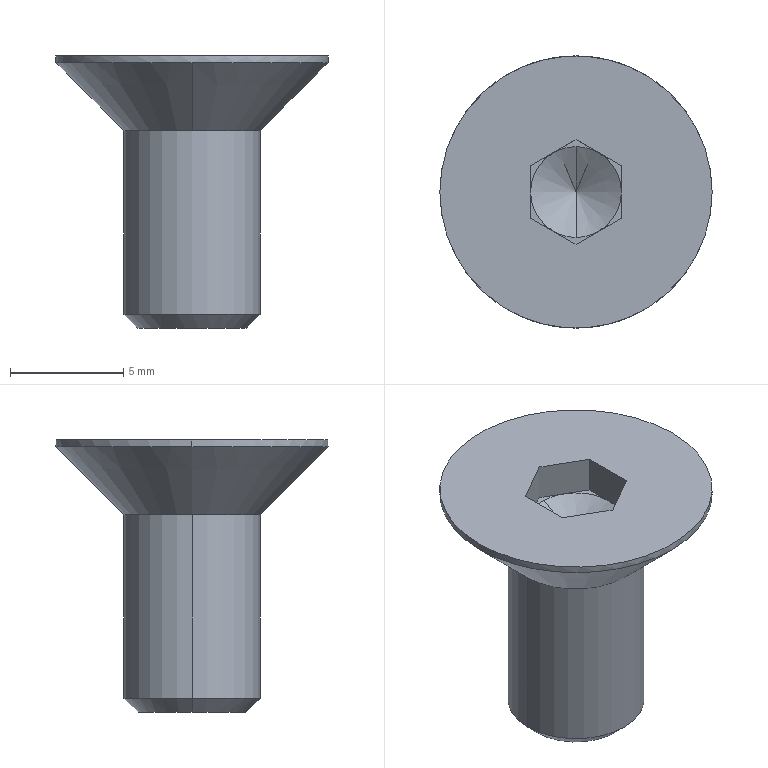Part | SolidWorks | features BaseBody 1 | 1 solid | 24 faces | box 12 x 12 x 12 mm | volume 446.831 mm3 | plane 14 | cone 6 | cylinder 4 | commonest cylinder face diameters 6 x2 12 x2
STEP:
#1=CARTESIAN_POINT('',(0.,6.,3.));
#2=VERTEX_POINT('',#1);
#3=CARTESIAN_POINT('',(-6.,0.,3.));
#4=VERTEX_POINT('',#3);
#5=CARTESIAN_POINT('',(0.,0.,3.));
#6=DIRECTION('',(0.,0.,1.));
#7=DIRECTION('',(1.,0.,0.));
#8=AXIS2_PLACEMENT_3D('',#5,#6,#7);
#9=CIRCLE('',#8,6.);
#10=EDGE_CURVE('',#2,#4,#9,.T.);
#11=ORIENTED_EDGE('',*,*,#10,.T.);
#12=CARTESIAN_POINT('',(-6.,0.,3.3));
#13=VERTEX_POINT('',#12);
#14=CARTESIAN_POINT('',(-6.,0.,0.));
#15=DIRECTION('',(0.,0.,1.));
#16=VECTOR('',#15,1000.);
#17=LINE('',#14,#16);
#18=EDGE_CURVE('',#4,#13,#17,.T.);
#19=ORIENTED_EDGE('',*,*,#18,.T.);
#20=CARTESIAN_POINT('',(6.,0.,3.3));
#21=VERTEX_POINT('',#20);
#22=CARTESIAN_POINT('',(0.,0.,3.3));
#23=DIRECTION('',(0.,0.,-1.));
#24=DIRECTION('',(1.,0.,0.));
#25=AXIS2_PLACEMENT_3D('',#22,#23,#24);
#26=CIRCLE('',#25,6.);
#27=EDGE_CURVE('',#13,#21,#26,.T.);
#28=ORIENTED_EDGE('',*,*,#27,.T.);
#29=CARTESIAN_POINT('',(6.,0.,3.));
#30=VERTEX_POINT('',#29);
#31=CARTESIAN_POINT('',(6.,0.,0.));
#32=DIRECTION('',(0.,0.,1.));
#33=VECTOR('',#32,1000.);
#34=LINE('',#31,#33);
#35=EDGE_CURVE('',#30,#21,#34,.T.);
#36=ORIENTED_EDGE('',*,*,#35,.F.);
#37=CARTESIAN_POINT('',(0.,0.,3.));
#38=DIRECTION('',(0.,0.,1.));
#39=DIRECTION('',(1.,0.,0.));
#40=AXIS2_PLACEMENT_3D('',#37,#38,#39);
#41=CIRCLE('',#40,6.);
#42=EDGE_CURVE('',#30,#2,#41,.T.);
#43=ORIENTED_EDGE('',*,*,#42,.T.);
#44=EDGE_LOOP('',(#11,#19,#28,#36,#43));
#45=FACE_OUTER_BOUND('',#44,.T.);
#46=CARTESIAN_POINT('',(0.,0.,0.));
#47=DIRECTION('',(0.,0.,1.));
#48=DIRECTION('',(1.,0.,0.));
#49=AXIS2_PLACEMENT_3D('',#46,#47,#48);
#50=CYLINDRICAL_SURFACE('',#49,6.);
#51=ADVANCED_FACE('',(#45),#50,.T.);
#52=CARTESIAN_POINT('',(3.,0.,0.));
#53=VERTEX_POINT('',#52);
#54=CARTESIAN_POINT('',(0.,3.,0.));
#55=VERTEX_POINT('',#54);
#56=CARTESIAN_POINT('',(0.,0.,0.));
#57=DIRECTION('',(0.,0.,1.));
#58=DIRECTION('',(1.,0.,0.));
#59=AXIS2_PLACEMENT_3D('',#56,#57,#58);
#60=CIRCLE('',#59,3.);
#61=EDGE_CURVE('',#53,#55,#60,.T.);
#62=ORIENTED_EDGE('',*,*,#61,.T.);
#63=CARTESIAN_POINT('',(0.,6.,3.));
#64=DIRECTION('',(0.,0.7071,0.7071));
#65=VECTOR('',#64,1000.);
#66=LINE('',#63,#65);
#67=EDGE_CURVE('',#55,#2,#66,.T.);
#68=ORIENTED_EDGE('',*,*,#67,.T.);
#69=ORIENTED_EDGE('',*,*,#42,.F.);
#70=CARTESIAN_POINT('',(0.,-6.,3.));
#71=VERTEX_POINT('',#70);
#72=CARTESIAN_POINT('',(0.,0.,3.));
#73=DIRECTION('',(0.,0.,1.));
#74=DIRECTION('',(1.,0.,0.));
#75=AXIS2_PLACEMENT_3D('',#72,#73,#74);
#76=CIRCLE('',#75,6.);
#77=EDGE_CURVE('',#71,#30,#76,.T.);
#78=ORIENTED_EDGE('',*,*,#77,.F.);
#79=CARTESIAN_POINT('',(0.,-3.,0.));
#80=VERTEX_POINT('',#79);
#81=CARTESIAN_POINT('',(0.,-6.,3.));
#82=DIRECTION('',(0.,-0.7071,0.7071));
#83=VECTOR('',#82,1000.);
#84=LINE('',#81,#83);
#85=EDGE_CURVE('',#80,#71,#84,.T.);
#86=ORIENTED_EDGE('',*,*,#85,.F.);
#87=CARTESIAN_POINT('',(0.,0.,0.));
#88=DIRECTION('',(0.,0.,1.));
#89=DIRECTION('',(1.,0.,0.));
#90=AXIS2_PLACEMENT_3D('',#87,#88,#89);
#91=CIRCLE('',#90,3.);
#92=EDGE_CURVE('',#80,#53,#91,.T.);
#93=ORIENTED_EDGE('',*,*,#92,.T.);
#94=EDGE_LOOP('',(#62,#68,#69,#78,#86,#93));
#95=FACE_OUTER_BOUND('',#94,.T.);
#96=CARTESIAN_POINT('',(0.,0.,3.));
#97=DIRECTION('',(0.,0.,1.));
#98=DIRECTION('',(0.,-1.,0.));
#99=AXIS2_PLACEMENT_3D('',#96,#97,#98);
#100=CONICAL_SURFACE('',#99,6.,0.7854);
#101=ADVANCED_FACE('',(#95),#100,.T.);
#102=CARTESIAN_POINT('',(3.,0.,-8.086));
#103=VERTEX_POINT('',#102);
#104=CARTESIAN_POINT('',(-3.,0.,-8.086));
#105=VERTEX_POINT('',#104);
#106=CARTESIAN_POINT('',(0.,0.,-8.086));
#107=DIRECTION('',(0.,0.,1.));
#108=DIRECTION('',(1.,0.,0.));
#109=AXIS2_PLACEMENT_3D('',#106,#107,#108);
#110=CIRCLE('',#109,3.);
#111=EDGE_CURVE('',#103,#105,#110,.T.);
#112=ORIENTED_EDGE('',*,*,#111,.T.);
#113=CARTESIAN_POINT('',(-3.,0.,0.));
#114=VERTEX_POINT('',#113);
#115=CARTESIAN_POINT('',(-3.,0.,-8.7));
#116=DIRECTION('',(0.,0.,1.));
#117=VECTOR('',#116,1000.);
#118=LINE('',#115,#117);
#119=EDGE_CURVE('',#105,#114,#118,.T.);
#120=ORIENTED_EDGE('',*,*,#119,.T.);
#121=CARTESIAN_POINT('',(0.,0.,0.));
#122=DIRECTION('',(0.,0.,1.));
#123=DIRECTION('',(1.,0.,0.));
#124=AXIS2_PLACEMENT_3D('',#121,#122,#123);
#125=CIRCLE('',#124,3.);
#126=EDGE_CURVE('',#55,#114,#125,.T.);
#127=ORIENTED_EDGE('',*,*,#126,.F.);
#128=ORIENTED_EDGE('',*,*,#61,.F.);
#129=CARTESIAN_POINT('',(3.,0.,-8.7));
#130=DIRECTION('',(0.,0.,1.));
#131=VECTOR('',#130,1000.);
#132=LINE('',#129,#131);
#133=EDGE_CURVE('',#103,#53,#132,.T.);
#134=ORIENTED_EDGE('',*,*,#133,.F.);
#135=EDGE_LOOP('',(#112,#120,#127,#128,#134));
#136=FACE_OUTER_BOUND('',#135,.T.);
#137=CARTESIAN_POINT('',(0.,0.,-8.7));
#138=DIRECTION('',(0.,0.,1.));
#139=DIRECTION('',(1.,0.,0.));
#140=AXIS2_PLACEMENT_3D('',#137,#138,#139);
#141=CYLINDRICAL_SURFACE('',#140,3.);
#142=ADVANCED_FACE('',(#136),#141,.T.);
#143=CARTESIAN_POINT('',(0.,0.,0.4953));
#144=VERTEX_POINT('',#143);
#145=CARTESIAN_POINT('',(0.,-2.,1.65));
#146=VERTEX_POINT('',#145);
#147=CARTESIAN_POINT('',(0.,-2.,1.65));
#148=DIRECTION('',(0.,-0.866,0.5));
#149=VECTOR('',#148,1000.);
#150=LINE('',#147,#149);
#151=EDGE_CURVE('',#144,#146,#150,.T.);
#152=ORIENTED_EDGE('',*,*,#151,.F.);
#153=CARTESIAN_POINT('',(0.,2.,1.65));
#154=VERTEX_POINT('',#153);
#155=CARTESIAN_POINT('',(0.,2.,1.65));
#156=DIRECTION('',(0.,0.866,0.5));
#157=VECTOR('',#156,1000.);
#158=LINE('',#155,#157);
#159=EDGE_CURVE('',#144,#154,#158,.T.);
#160=ORIENTED_EDGE('',*,*,#159,.T.);
#161=CARTESIAN_POINT('',(-1.,1.732,1.65));
#162=VERTEX_POINT('',#161);
#163=CARTESIAN_POINT('',(0.,0.,1.65));
#164=DIRECTION('',(0.,0.,-1.));
#165=DIRECTION('',(0.,-1.,0.));
#166=AXIS2_PLACEMENT_3D('',#163,#164,#165);
#167=CIRCLE('',#166,2.);
#168=EDGE_CURVE('',#162,#154,#167,.T.);
#169=ORIENTED_EDGE('',*,*,#168,.F.);
#170=CARTESIAN_POINT('',(-2.,0.,1.65));
#171=VERTEX_POINT('',#170);
#172=CARTESIAN_POINT('',(0.,0.,1.65));
#173=DIRECTION('',(0.,0.,-1.));
#174=DIRECTION('',(0.,-1.,0.));
#175=AXIS2_PLACEMENT_3D('',#172,#173,#174);
#176=CIRCLE('',#175,2.);
#177=EDGE_CURVE('',#171,#162,#176,.T.);
#178=ORIENTED_EDGE('',*,*,#177,.F.);
#179=CARTESIAN_POINT('',(-1.,-1.732,1.65));
#180=VERTEX_POINT('',#179);
#181=CARTESIAN_POINT('',(0.,0.,1.65));
#182=DIRECTION('',(0.,0.,-1.));
#183=DIRECTION('',(0.,-1.,0.));
#184=AXIS2_PLACEMENT_3D('',#181,#182,#183);
#185=CIRCLE('',#184,2.);
#186=EDGE_CURVE('',#180,#171,#185,.T.);
#187=ORIENTED_EDGE('',*,*,#186,.F.);
#188=CARTESIAN_POINT('',(0.,0.,1.65));
#189=DIRECTION('',(0.,0.,-1.));
#190=DIRECTION('',(0.,-1.,0.));
#191=AXIS2_PLACEMENT_3D('',#188,#189,#190);
#192=CIRCLE('',#191,2.);
#193=EDGE_CURVE('',#146,#180,#192,.T.);
#194=ORIENTED_EDGE('',*,*,#193,.F.);
#195=EDGE_LOOP('',(#152,#160,#169,#178,#187,#194));
#196=FACE_OUTER_BOUND('',#195,.T.);
#197=CARTESIAN_POINT('',(0.,0.,1.65));
#198=DIRECTION('',(0.,0.,1.));
#199=DIRECTION('',(0.,-1.,0.));
#200=AXIS2_PLACEMENT_3D('',#197,#198,#199);
#201=CONICAL_SURFACE('',#200,2.,1.047);
#202=ADVANCED_FACE('',(#196),#201,.F.);
#203=CARTESIAN_POINT('',(2.387,0.,-8.7));
#204=VERTEX_POINT('',#203);
#205=CARTESIAN_POINT('',(-2.387,0.,-8.7));
#206=VERTEX_POINT('',#205);
#207=CARTESIAN_POINT('',(0.,0.,-8.7));
#208=DIRECTION('',(0.,0.,1.));
#209=DIRECTION('',(1.,0.,0.));
#210=AXIS2_PLACEMENT_3D('',#207,#208,#209);
#211=CIRCLE('',#210,2.387);
#212=EDGE_CURVE('',#204,#206,#211,.T.);
#213=ORIENTED_EDGE('',*,*,#212,.T.);
#214=CARTESIAN_POINT('',(-3.,0.,-8.087));
#215=DIRECTION('',(-0.7071,0.,0.7071));
#216=VECTOR('',#215,1000.);
#217=LINE('',#214,#216);
#218=EDGE_CURVE('',#206,#105,#217,.T.);
#219=ORIENTED_EDGE('',*,*,#218,.T.);
#220=ORIENTED_EDGE('',*,*,#111,.F.);
#221=CARTESIAN_POINT('',(3.,0.,-8.087));
#222=DIRECTION('',(0.7071,0.,0.7071));
#223=VECTOR('',#222,1000.);
#224=LINE('',#221,#223);
#225=EDGE_CURVE('',#204,#103,#224,.T.);
#226=ORIENTED_EDGE('',*,*,#225,.F.);
#227=EDGE_LOOP('',(#213,#219,#220,#226));
#228=FACE_OUTER_BOUND('',#227,.T.);
#229=CARTESIAN_POINT('',(0.,0.,-8.087));
#230=DIRECTION('',(0.,0.,1.));
#231=DIRECTION('',(1.,0.,0.));
#232=AXIS2_PLACEMENT_3D('',#229,#230,#231);
#233=CONICAL_SURFACE('',#232,3.,0.7854);
#234=ADVANCED_FACE('',(#228),#233,.T.);
#235=CARTESIAN_POINT('',(0.,0.,3.3));
#236=DIRECTION('',(0.,0.,-1.));
#237=DIRECTION('',(1.,0.,0.));
#238=AXIS2_PLACEMENT_3D('',#235,#236,#237);
#239=CIRCLE('',#238,6.);
#240=EDGE_CURVE('',#21,#13,#239,.T.);
#241=ORIENTED_EDGE('',*,*,#240,.F.);
#242=ORIENTED_EDGE('',*,*,#27,.F.);
#243=EDGE_LOOP('',(#241,#242));
#244=FACE_OUTER_BOUND('',#243,.T.);
#245=CARTESIAN_POINT('',(-2.,1.155,3.3));
#246=VERTEX_POINT('',#245);
#247=CARTESIAN_POINT('',(-2.,-1.155,3.3));
#248=VERTEX_POINT('',#247);
#249=CARTESIAN_POINT('',(-2.,0.,3.3));
#250=DIRECTION('',(0.,-1.,0.));
#251=VECTOR('',#250,1000.);
#252=LINE('',#249,#251);
#253=EDGE_CURVE('',#246,#248,#252,.T.);
#254=ORIENTED_EDGE('',*,*,#253,.F.);
#255=CARTESIAN_POINT('',(0.,2.309,3.3));
#256=VERTEX_POINT('',#255);
#257=CARTESIAN_POINT('',(0.,2.309,3.3));
#258=DIRECTION('',(-0.866,-0.5,0.));
#259=VECTOR('',#258,1000.);
#260=LINE('',#257,#259);
#261=EDGE_CURVE('',#256,#246,#260,.T.);
#262=ORIENTED_EDGE('',*,*,#261,.F.);
#263=CARTESIAN_POINT('',(2.,1.155,3.3));
#264=VERTEX_POINT('',#263);
#265=CARTESIAN_POINT('',(2.,1.155,3.3));
#266=DIRECTION('',(-0.866,0.5,0.));
#267=VECTOR('',#266,1000.);
#268=LINE('',#265,#267);
#269=EDGE_CURVE('',#264,#256,#268,.T.);
#270=ORIENTED_EDGE('',*,*,#269,.F.);
#271=CARTESIAN_POINT('',(2.,-1.155,3.3));
#272=VERTEX_POINT('',#271);
#273=CARTESIAN_POINT('',(2.,0.,3.3));
#274=DIRECTION('',(0.,1.,0.));
#275=VECTOR('',#274,1000.);
#276=LINE('',#273,#275);
#277=EDGE_CURVE('',#272,#264,#276,.T.);
#278=ORIENTED_EDGE('',*,*,#277,.F.);
#279=CARTESIAN_POINT('',(0.,-2.309,3.3));
#280=VERTEX_POINT('',#279);
#281=CARTESIAN_POINT('',(0.,-2.309,3.3));
#282=DIRECTION('',(0.866,0.5,0.));
#283=VECTOR('',#282,1000.);
#284=LINE('',#281,#283);
#285=EDGE_CURVE('',#280,#272,#284,.T.);
#286=ORIENTED_EDGE('',*,*,#285,.F.);
#287=CARTESIAN_POINT('',(-2.,-1.155,3.3));
#288=DIRECTION('',(0.866,-0.5,0.));
#289=VECTOR('',#288,1000.);
#290=LINE('',#287,#289);
#291=EDGE_CURVE('',#248,#280,#290,.T.);
#292=ORIENTED_EDGE('',*,*,#291,.F.);
#293=EDGE_LOOP('',(#254,#262,#270,#278,#286,#292));
#294=FACE_BOUND('',#293,.T.);
#295=CARTESIAN_POINT('',(0.,0.,3.3));
#296=DIRECTION('',(0.,0.,-1.));
#297=DIRECTION('',(-1.,0.,0.));
#298=AXIS2_PLACEMENT_3D('',#295,#296,#297);
#299=PLANE('',#298);
#300=ADVANCED_FACE('',(#244,#294),#299,.F.);
#301=ORIENTED_EDGE('',*,*,#18,.F.);
#302=CARTESIAN_POINT('',(0.,0.,3.));
#303=DIRECTION('',(0.,0.,1.));
#304=DIRECTION('',(1.,0.,0.));
#305=AXIS2_PLACEMENT_3D('',#302,#303,#304);
#306=CIRCLE('',#305,6.);
#307=EDGE_CURVE('',#4,#71,#306,.T.);
#308=ORIENTED_EDGE('',*,*,#307,.T.);
#309=ORIENTED_EDGE('',*,*,#77,.T.);
#310=ORIENTED_EDGE('',*,*,#35,.T.);
#311=ORIENTED_EDGE('',*,*,#240,.T.);
#312=EDGE_LOOP('',(#301,#308,#309,#310,#311));
#313=FACE_OUTER_BOUND('',#312,.T.);
#314=CARTESIAN_POINT('',(0.,0.,0.));
#315=DIRECTION('',(0.,0.,1.));
#316=DIRECTION('',(1.,0.,0.));
#317=AXIS2_PLACEMENT_3D('',#314,#315,#316);
#318=CYLINDRICAL_SURFACE('',#317,6.);
#319=ADVANCED_FACE('',(#313),#318,.T.);
#320=CARTESIAN_POINT('',(0.,-2.309,1.65));
#321=VERTEX_POINT('',#320);
#322=CARTESIAN_POINT('',(-2.,-1.155,1.65));
#323=DIRECTION('',(0.866,-0.5,0.));
#324=VECTOR('',#323,1000.);
#325=LINE('',#322,#324);
#326=EDGE_CURVE('',#180,#321,#325,.T.);
#327=ORIENTED_EDGE('',*,*,#326,.F.);
#328=CARTESIAN_POINT('',(-2.,-1.155,1.65));
#329=VERTEX_POINT('',#328);
#330=CARTESIAN_POINT('',(-2.,-1.155,1.65));
#331=DIRECTION('',(0.866,-0.5,0.));
#332=VECTOR('',#331,1000.);
#333=LINE('',#330,#332);
#334=EDGE_CURVE('',#329,#180,#333,.T.);
#335=ORIENTED_EDGE('',*,*,#334,.F.);
#336=CARTESIAN_POINT('',(-2.,-1.155,1.65));
#337=DIRECTION('',(0.,0.,-1.));
#338=VECTOR('',#337,1000.);
#339=LINE('',#336,#338);
#340=EDGE_CURVE('',#248,#329,#339,.T.);
#341=ORIENTED_EDGE('',*,*,#340,.F.);
#342=ORIENTED_EDGE('',*,*,#291,.T.);
#343=CARTESIAN_POINT('',(0.,-2.309,1.65));
#344=DIRECTION('',(0.,0.,1.));
#345=VECTOR('',#344,1000.);
#346=LINE('',#343,#345);
#347=EDGE_CURVE('',#321,#280,#346,.T.);
#348=ORIENTED_EDGE('',*,*,#347,.F.);
#349=EDGE_LOOP('',(#327,#335,#341,#342,#348));
#350=FACE_OUTER_BOUND('',#349,.T.);
#351=CARTESIAN_POINT('',(-2.,-1.155,1.65));
#352=DIRECTION('',(-0.5,-0.866,0.));
#353=DIRECTION('',(0.866,-0.5,0.));
#354=AXIS2_PLACEMENT_3D('',#351,#352,#353);
#355=PLANE('',#354);
#356=ADVANCED_FACE('',(#350),#355,.F.);
#357=CARTESIAN_POINT('',(-2.,0.,1.65));
#358=DIRECTION('',(0.,-1.,0.));
#359=VECTOR('',#358,1000.);
#360=LINE('',#357,#359);
#361=EDGE_CURVE('',#171,#329,#360,.T.);
#362=ORIENTED_EDGE('',*,*,#361,.F.);
#363=CARTESIAN_POINT('',(-2.,1.155,1.65));
#364=VERTEX_POINT('',#363);
#365=CARTESIAN_POINT('',(-2.,0.,1.65));
#366=DIRECTION('',(0.,-1.,0.));
#367=VECTOR('',#366,1000.);
#368=LINE('',#365,#367);
#369=EDGE_CURVE('',#364,#171,#368,.T.);
#370=ORIENTED_EDGE('',*,*,#369,.F.);
#371=CARTESIAN_POINT('',(-2.,1.155,1.65));
#372=DIRECTION('',(0.,0.,-1.));
#373=VECTOR('',#372,1000.);
#374=LINE('',#371,#373);
#375=EDGE_CURVE('',#246,#364,#374,.T.);
#376=ORIENTED_EDGE('',*,*,#375,.F.);
#377=ORIENTED_EDGE('',*,*,#253,.T.);
#378=ORIENTED_EDGE('',*,*,#340,.T.);
#379=EDGE_LOOP('',(#362,#370,#376,#377,#378));
#380=FACE_OUTER_BOUND('',#379,.T.);
#381=CARTESIAN_POINT('',(-2.,1.155,1.65));
#382=DIRECTION('',(-1.,0.,0.));
#383=DIRECTION('',(0.,0.,1.));
#384=AXIS2_PLACEMENT_3D('',#381,#382,#383);
#385=PLANE('',#384);
#386=ADVANCED_FACE('',(#380),#385,.F.);
#387=CARTESIAN_POINT('',(-1.,1.732,1.65));
#388=DIRECTION('',(-0.866,-0.5,0.));
#389=VECTOR('',#388,1000.);
#390=LINE('',#387,#389);
#391=EDGE_CURVE('',#162,#364,#390,.T.);
#392=ORIENTED_EDGE('',*,*,#391,.F.);
#393=CARTESIAN_POINT('',(0.,2.309,1.65));
#394=VERTEX_POINT('',#393);
#395=CARTESIAN_POINT('',(0.,2.309,1.65));
#396=DIRECTION('',(-0.866,-0.5,0.));
#397=VECTOR('',#396,1000.);
#398=LINE('',#395,#397);
#399=EDGE_CURVE('',#394,#162,#398,.T.);
#400=ORIENTED_EDGE('',*,*,#399,.F.);
#401=CARTESIAN_POINT('',(0.,2.309,1.65));
#402=DIRECTION('',(0.,0.,-1.));
#403=VECTOR('',#402,1000.);
#404=LINE('',#401,#403);
#405=EDGE_CURVE('',#256,#394,#404,.T.);
#406=ORIENTED_EDGE('',*,*,#405,.F.);
#407=ORIENTED_EDGE('',*,*,#261,.T.);
#408=ORIENTED_EDGE('',*,*,#375,.T.);
#409=EDGE_LOOP('',(#392,#400,#406,#407,#408));
#410=FACE_OUTER_BOUND('',#409,.T.);
#411=CARTESIAN_POINT('',(0.,2.309,1.65));
#412=DIRECTION('',(-0.5,0.866,0.));
#413=DIRECTION('',(-0.866,-0.5,0.));
#414=AXIS2_PLACEMENT_3D('',#411,#412,#413);
#415=PLANE('',#414);
#416=ADVANCED_FACE('',(#410),#415,.F.);
#417=CARTESIAN_POINT('',(1.,1.732,1.65));
#418=VERTEX_POINT('',#417);
#419=CARTESIAN_POINT('',(1.,1.732,1.65));
#420=DIRECTION('',(-0.866,0.5,0.));
#421=VECTOR('',#420,1000.);
#422=LINE('',#419,#421);
#423=EDGE_CURVE('',#418,#394,#422,.T.);
#424=ORIENTED_EDGE('',*,*,#423,.F.);
#425=CARTESIAN_POINT('',(2.,1.155,1.65));
#426=VERTEX_POINT('',#425);
#427=CARTESIAN_POINT('',(2.,1.155,1.65));
#428=DIRECTION('',(-0.866,0.5,0.));
#429=VECTOR('',#428,1000.);
#430=LINE('',#427,#429);
#431=EDGE_CURVE('',#426,#418,#430,.T.);
#432=ORIENTED_EDGE('',*,*,#431,.F.);
#433=CARTESIAN_POINT('',(2.,1.155,1.65));
#434=DIRECTION('',(0.,0.,-1.));
#435=VECTOR('',#434,1000.);
#436=LINE('',#433,#435);
#437=EDGE_CURVE('',#264,#426,#436,.T.);
#438=ORIENTED_EDGE('',*,*,#437,.F.);
#439=ORIENTED_EDGE('',*,*,#269,.T.);
#440=ORIENTED_EDGE('',*,*,#405,.T.);
#441=EDGE_LOOP('',(#424,#432,#438,#439,#440));
#442=FACE_OUTER_BOUND('',#441,.T.);
#443=CARTESIAN_POINT('',(2.,1.155,1.65));
#444=DIRECTION('',(0.5,0.866,0.));
#445=DIRECTION('',(-0.866,0.5,0.));
#446=AXIS2_PLACEMENT_3D('',#443,#444,#445);
#447=PLANE('',#446);
#448=ADVANCED_FACE('',(#442),#447,.F.);
#449=CARTESIAN_POINT('',(2.,0.,1.65));
#450=VERTEX_POINT('',#449);
#451=CARTESIAN_POINT('',(2.,0.,1.65));
#452=DIRECTION('',(0.,1.,0.));
#453=VECTOR('',#452,1000.);
#454=LINE('',#451,#453);
#455=EDGE_CURVE('',#450,#426,#454,.T.);
#456=ORIENTED_EDGE('',*,*,#455,.F.);
#457=CARTESIAN_POINT('',(2.,-1.155,1.65));
#458=VERTEX_POINT('',#457);
#459=CARTESIAN_POINT('',(2.,0.,1.65));
#460=DIRECTION('',(0.,1.,0.));
#461=VECTOR('',#460,1000.);
#462=LINE('',#459,#461);
#463=EDGE_CURVE('',#458,#450,#462,.T.);
#464=ORIENTED_EDGE('',*,*,#463,.F.);
#465=CARTESIAN_POINT('',(2.,-1.155,1.65));
#466=DIRECTION('',(0.,0.,-1.));
#467=VECTOR('',#466,1000.);
#468=LINE('',#465,#467);
#469=EDGE_CURVE('',#272,#458,#468,.T.);
#470=ORIENTED_EDGE('',*,*,#469,.F.);
#471=ORIENTED_EDGE('',*,*,#277,.T.);
#472=ORIENTED_EDGE('',*,*,#437,.T.);
#473=EDGE_LOOP('',(#456,#464,#470,#471,#472));
#474=FACE_OUTER_BOUND('',#473,.T.);
#475=CARTESIAN_POINT('',(2.,-1.155,1.65));
#476=DIRECTION('',(1.,0.,0.));
#477=DIRECTION('',(0.,0.,-1.));
#478=AXIS2_PLACEMENT_3D('',#475,#476,#477);
#479=PLANE('',#478);
#480=ADVANCED_FACE('',(#474),#479,.F.);
#481=CARTESIAN_POINT('',(1.,-1.732,1.65));
#482=VERTEX_POINT('',#481);
#483=CARTESIAN_POINT('',(1.,-1.732,1.65));
#484=DIRECTION('',(0.866,0.5,0.));
#485=VECTOR('',#484,1000.);
#486=LINE('',#483,#485);
#487=EDGE_CURVE('',#482,#458,#486,.T.);
#488=ORIENTED_EDGE('',*,*,#487,.F.);
#489=CARTESIAN_POINT('',(0.,-2.309,1.65));
#490=DIRECTION('',(0.866,0.5,0.));
#491=VECTOR('',#490,1000.);
#492=LINE('',#489,#491);
#493=EDGE_CURVE('',#321,#482,#492,.T.);
#494=ORIENTED_EDGE('',*,*,#493,.F.);
#495=ORIENTED_EDGE('',*,*,#347,.T.);
#496=ORIENTED_EDGE('',*,*,#285,.T.);
#497=ORIENTED_EDGE('',*,*,#469,.T.);
#498=EDGE_LOOP('',(#488,#494,#495,#496,#497));
#499=FACE_OUTER_BOUND('',#498,.T.);
#500=CARTESIAN_POINT('',(0.,-2.309,1.65));
#501=DIRECTION('',(0.5,-0.866,0.));
#502=DIRECTION('',(0.866,0.5,0.));
#503=AXIS2_PLACEMENT_3D('',#500,#501,#502);
#504=PLANE('',#503);
#505=ADVANCED_FACE('',(#499),#504,.F.);
#506=ORIENTED_EDGE('',*,*,#67,.F.);
#507=ORIENTED_EDGE('',*,*,#126,.T.);
#508=CARTESIAN_POINT('',(0.,0.,0.));
#509=DIRECTION('',(0.,0.,1.));
#510=DIRECTION('',(1.,0.,0.));
#511=AXIS2_PLACEMENT_3D('',#508,#509,#510);
#512=CIRCLE('',#511,3.);
#513=EDGE_CURVE('',#114,#80,#512,.T.);
#514=ORIENTED_EDGE('',*,*,#513,.T.);
#515=ORIENTED_EDGE('',*,*,#85,.T.);
#516=ORIENTED_EDGE('',*,*,#307,.F.);
#517=ORIENTED_EDGE('',*,*,#10,.F.);
#518=EDGE_LOOP('',(#506,#507,#514,#515,#516,#517));
#519=FACE_OUTER_BOUND('',#518,.T.);
#520=CARTESIAN_POINT('',(0.,0.,3.));
#521=DIRECTION('',(0.,0.,1.));
#522=DIRECTION('',(0.,-1.,0.));
#523=AXIS2_PLACEMENT_3D('',#520,#521,#522);
#524=CONICAL_SURFACE('',#523,6.,0.7854);
#525=ADVANCED_FACE('',(#519),#524,.T.);
#526=ORIENTED_EDGE('',*,*,#326,.T.);
#527=ORIENTED_EDGE('',*,*,#493,.T.);
#528=CARTESIAN_POINT('',(0.,0.,1.65));
#529=DIRECTION('',(0.,0.,-1.));
#530=DIRECTION('',(0.,-1.,0.));
#531=AXIS2_PLACEMENT_3D('',#528,#529,#530);
#532=CIRCLE('',#531,2.);
#533=EDGE_CURVE('',#482,#146,#532,.T.);
#534=ORIENTED_EDGE('',*,*,#533,.T.);
#535=ORIENTED_EDGE('',*,*,#193,.T.);
#536=EDGE_LOOP('',(#526,#527,#534,#535));
#537=FACE_OUTER_BOUND('',#536,.T.);
#538=CARTESIAN_POINT('',(0.,0.,1.65));
#539=DIRECTION('',(0.,0.,1.));
#540=DIRECTION('',(1.,0.,0.));
#541=AXIS2_PLACEMENT_3D('',#538,#539,#540);
#542=PLANE('',#541);
#543=ADVANCED_FACE('',(#537),#542,.T.);
#544=ORIENTED_EDGE('',*,*,#119,.F.);
#545=CARTESIAN_POINT('',(0.,0.,-8.086));
#546=DIRECTION('',(0.,0.,1.));
#547=DIRECTION('',(1.,0.,0.));
#548=AXIS2_PLACEMENT_3D('',#545,#546,#547);
#549=CIRCLE('',#548,3.);
#550=EDGE_CURVE('',#105,#103,#549,.T.);
#551=ORIENTED_EDGE('',*,*,#550,.T.);
#552=ORIENTED_EDGE('',*,*,#133,.T.);
#553=ORIENTED_EDGE('',*,*,#92,.F.);
#554=ORIENTED_EDGE('',*,*,#513,.F.);
#555=EDGE_LOOP('',(#544,#551,#552,#553,#554));
#556=FACE_OUTER_BOUND('',#555,.T.);
#557=CARTESIAN_POINT('',(0.,0.,-8.7));
#558=DIRECTION('',(0.,0.,1.));
#559=DIRECTION('',(1.,0.,0.));
#560=AXIS2_PLACEMENT_3D('',#557,#558,#559);
#561=CYLINDRICAL_SURFACE('',#560,3.);
#562=ADVANCED_FACE('',(#556),#561,.T.);
#563=ORIENTED_EDGE('',*,*,#159,.F.);
#564=ORIENTED_EDGE('',*,*,#151,.T.);
#565=ORIENTED_EDGE('',*,*,#533,.F.);
#566=CARTESIAN_POINT('',(0.,0.,1.65));
#567=DIRECTION('',(0.,0.,-1.));
#568=DIRECTION('',(0.,-1.,0.));
#569=AXIS2_PLACEMENT_3D('',#566,#567,#568);
#570=CIRCLE('',#569,2.);
#571=EDGE_CURVE('',#450,#482,#570,.T.);
#572=ORIENTED_EDGE('',*,*,#571,.F.);
#573=CARTESIAN_POINT('',(0.,0.,1.65));
#574=DIRECTION('',(0.,0.,-1.));
#575=DIRECTION('',(0.,-1.,0.));
#576=AXIS2_PLACEMENT_3D('',#573,#574,#575);
#577=CIRCLE('',#576,2.);
#578=EDGE_CURVE('',#418,#450,#577,.T.);
#579=ORIENTED_EDGE('',*,*,#578,.F.);
#580=CARTESIAN_POINT('',(0.,0.,1.65));
#581=DIRECTION('',(0.,0.,-1.));
#582=DIRECTION('',(0.,-1.,0.));
#583=AXIS2_PLACEMENT_3D('',#580,#581,#582);
#584=CIRCLE('',#583,2.);
#585=EDGE_CURVE('',#154,#418,#584,.T.);
#586=ORIENTED_EDGE('',*,*,#585,.F.);
#587=EDGE_LOOP('',(#563,#564,#565,#572,#579,#586));
#588=FACE_OUTER_BOUND('',#587,.T.);
#589=CARTESIAN_POINT('',(0.,0.,1.65));
#590=DIRECTION('',(0.,0.,1.));
#591=DIRECTION('',(0.,-1.,0.));
#592=AXIS2_PLACEMENT_3D('',#589,#590,#591);
#593=CONICAL_SURFACE('',#592,2.,1.047);
#594=ADVANCED_FACE('',(#588),#593,.F.);
#595=ORIENTED_EDGE('',*,*,#218,.F.);
#596=CARTESIAN_POINT('',(0.,0.,-8.7));
#597=DIRECTION('',(0.,0.,1.));
#598=DIRECTION('',(1.,0.,0.));
#599=AXIS2_PLACEMENT_3D('',#596,#597,#598);
#600=CIRCLE('',#599,2.387);
#601=EDGE_CURVE('',#206,#204,#600,.T.);
#602=ORIENTED_EDGE('',*,*,#601,.T.);
#603=ORIENTED_EDGE('',*,*,#225,.T.);
#604=ORIENTED_EDGE('',*,*,#550,.F.);
#605=EDGE_LOOP('',(#595,#602,#603,#604));
#606=FACE_OUTER_BOUND('',#605,.T.);
#607=CARTESIAN_POINT('',(0.,0.,-8.087));
#608=DIRECTION('',(0.,0.,1.));
#609=DIRECTION('',(1.,0.,0.));
#610=AXIS2_PLACEMENT_3D('',#607,#608,#609);
#611=CONICAL_SURFACE('',#610,3.,0.7854);
#612=ADVANCED_FACE('',(#606),#611,.T.);
#613=ORIENTED_EDGE('',*,*,#361,.T.);
#614=ORIENTED_EDGE('',*,*,#334,.T.);
#615=ORIENTED_EDGE('',*,*,#186,.T.);
#616=EDGE_LOOP('',(#613,#614,#615));
#617=FACE_OUTER_BOUND('',#616,.T.);
#618=CARTESIAN_POINT('',(0.,0.,1.65));
#619=DIRECTION('',(0.,0.,1.));
#620=DIRECTION('',(1.,0.,0.));
#621=AXIS2_PLACEMENT_3D('',#618,#619,#620);
#622=PLANE('',#621);
#623=ADVANCED_FACE('',(#617),#622,.T.);
#624=ORIENTED_EDGE('',*,*,#487,.T.);
#625=ORIENTED_EDGE('',*,*,#463,.T.);
#626=ORIENTED_EDGE('',*,*,#571,.T.);
#627=EDGE_LOOP('',(#624,#625,#626));
#628=FACE_OUTER_BOUND('',#627,.T.);
#629=CARTESIAN_POINT('',(0.,0.,1.65));
#630=DIRECTION('',(0.,0.,1.));
#631=DIRECTION('',(1.,0.,0.));
#632=AXIS2_PLACEMENT_3D('',#629,#630,#631);
#633=PLANE('',#632);
#634=ADVANCED_FACE('',(#628),#633,.T.);
#635=ORIENTED_EDGE('',*,*,#212,.F.);
#636=ORIENTED_EDGE('',*,*,#601,.F.);
#637=EDGE_LOOP('',(#635,#636));
#638=FACE_OUTER_BOUND('',#637,.T.);
#639=CARTESIAN_POINT('',(0.,2.386,-8.7));
#640=DIRECTION('',(0.,0.,1.));
#641=DIRECTION('',(1.,0.,0.));
#642=AXIS2_PLACEMENT_3D('',#639,#640,#641);
#643=PLANE('',#642);
#644=ADVANCED_FACE('',(#638),#643,.F.);
#645=ORIENTED_EDGE('',*,*,#455,.T.);
#646=ORIENTED_EDGE('',*,*,#431,.T.);
#647=ORIENTED_EDGE('',*,*,#578,.T.);
#648=EDGE_LOOP('',(#645,#646,#647));
#649=FACE_OUTER_BOUND('',#648,.T.);
#650=CARTESIAN_POINT('',(0.,0.,1.65));
#651=DIRECTION('',(0.,0.,1.));
#652=DIRECTION('',(1.,0.,0.));
#653=AXIS2_PLACEMENT_3D('',#650,#651,#652);
#654=PLANE('',#653);
#655=ADVANCED_FACE('',(#649),#654,.T.);
#656=ORIENTED_EDGE('',*,*,#423,.T.);
#657=ORIENTED_EDGE('',*,*,#399,.T.);
#658=ORIENTED_EDGE('',*,*,#168,.T.);
#659=ORIENTED_EDGE('',*,*,#585,.T.);
#660=EDGE_LOOP('',(#656,#657,#658,#659));
#661=FACE_OUTER_BOUND('',#660,.T.);
#662=CARTESIAN_POINT('',(0.,0.,1.65));
#663=DIRECTION('',(0.,0.,1.));
#664=DIRECTION('',(1.,0.,0.));
#665=AXIS2_PLACEMENT_3D('',#662,#663,#664);
#666=PLANE('',#665);
#667=ADVANCED_FACE('',(#661),#666,.T.);
#668=ORIENTED_EDGE('',*,*,#391,.T.);
#669=ORIENTED_EDGE('',*,*,#369,.T.);
#670=ORIENTED_EDGE('',*,*,#177,.T.);
#671=EDGE_LOOP('',(#668,#669,#670));
#672=FACE_OUTER_BOUND('',#671,.T.);
#673=CARTESIAN_POINT('',(0.,0.,1.65));
#674=DIRECTION('',(0.,0.,1.));
#675=DIRECTION('',(1.,0.,0.));
#676=AXIS2_PLACEMENT_3D('',#673,#674,#675);
#677=PLANE('',#676);
#678=ADVANCED_FACE('',(#672),#677,.T.);
#679=CLOSED_SHELL('',(#51,#101,#142,#202,#234,#300,#319,#356,#386,#416,#448,#480,#505,#525,#543,#562,#594,#612,#623,#634,#644,#655,#667,#678));
#680=MANIFOLD_SOLID_BREP('',#679);
#681=CARTESIAN_POINT('',(0.,0.,0.));
#682=DIRECTION('',(0.,0.,1.));
#683=DIRECTION('',(1.,0.,0.));
#684=AXIS2_PLACEMENT_3D('',#681,#682,#683);
#685=(LENGTH_UNIT()NAMED_UNIT(*)SI_UNIT(.MILLI.,.METRE.));
#686=UNCERTAINTY_MEASURE_WITH_UNIT(LENGTH_MEASURE(0.00001),#685,'','');
#687=(NAMED_UNIT(*)PLANE_ANGLE_UNIT()SI_UNIT($,.RADIAN.));
#688=(NAMED_UNIT(*)SI_UNIT($,.STERADIAN.)SOLID_ANGLE_UNIT());
#689=(GEOMETRIC_REPRESENTATION_CONTEXT(3)GLOBAL_UNCERTAINTY_ASSIGNED_CONTEXT((#686))GLOBAL_UNIT_ASSIGNED_CONTEXT((#685,#687,#688))REPRESENTATION_CONTEXT('',''));
#690=ADVANCED_BREP_SHAPE_REPRESENTATION('',(#680,#684),#689);